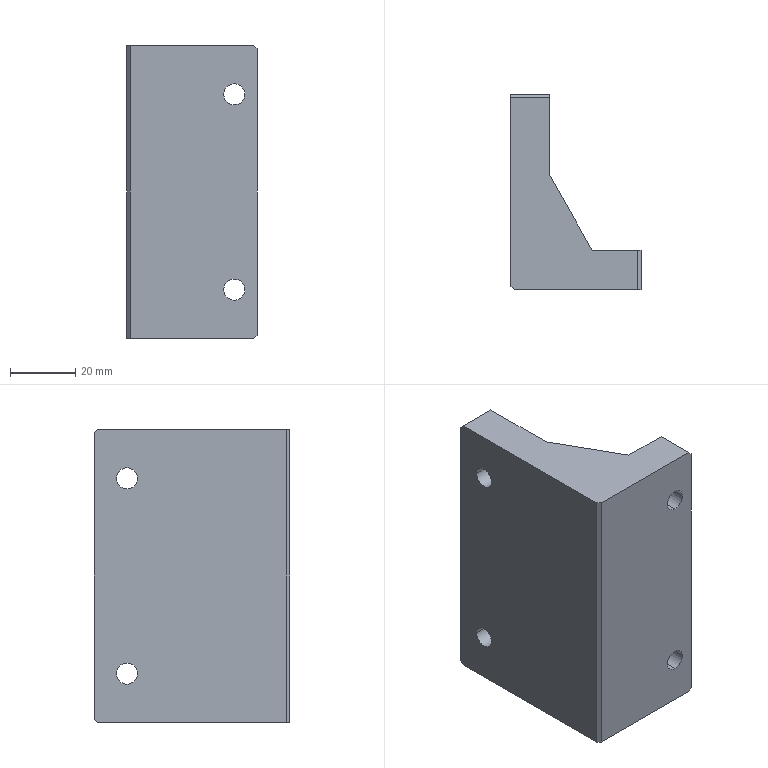Part | NX | features BREP 1 | 1 solid | 22 faces | box 40 x 60 x 90 mm | volume 106833 mm3 | plane 14 | cylinder 8 | commonest cylinder face diameters 6.5 x8
STEP:
#1=CARTESIAN_POINT('',(0.,46.75,75.));
#2=VERTEX_POINT('',#1);
#3=CARTESIAN_POINT('',(0.,53.25,75.));
#4=VERTEX_POINT('',#3);
#5=CARTESIAN_POINT('',(0.,50.,75.));
#6=DIRECTION('',(1.,0.,0.));
#7=DIRECTION('',(0.,0.,-1.));
#8=AXIS2_PLACEMENT_3D('',#5,#6,#7);
#9=CIRCLE('',#8,3.25);
#10=EDGE_CURVE('',#2,#4,#9,.T.);
#11=ORIENTED_EDGE('',*,*,#10,.F.);
#12=CARTESIAN_POINT('',(12.,46.75,75.));
#13=VERTEX_POINT('',#12);
#14=CARTESIAN_POINT('',(-18.,46.75,75.));
#15=DIRECTION('',(1.,0.,0.));
#16=VECTOR('',#15,1000.);
#17=LINE('',#14,#16);
#18=EDGE_CURVE('',#13,#2,#17,.F.);
#19=ORIENTED_EDGE('',*,*,#18,.F.);
#20=CARTESIAN_POINT('',(12.,53.25,75.));
#21=VERTEX_POINT('',#20);
#22=CARTESIAN_POINT('',(12.,50.,75.));
#23=DIRECTION('',(1.,0.,0.));
#24=DIRECTION('',(0.,1.,0.));
#25=AXIS2_PLACEMENT_3D('',#22,#23,#24);
#26=CIRCLE('',#25,3.25);
#27=EDGE_CURVE('',#13,#21,#26,.T.);
#28=ORIENTED_EDGE('',*,*,#27,.T.);
#29=CARTESIAN_POINT('',(-18.,53.25,75.));
#30=DIRECTION('',(1.,0.,0.));
#31=VECTOR('',#30,1000.);
#32=LINE('',#29,#31);
#33=EDGE_CURVE('',#21,#4,#32,.F.);
#34=ORIENTED_EDGE('',*,*,#33,.T.);
#35=EDGE_LOOP('',(#11,#19,#28,#34));
#36=FACE_BOUND('',#35,.T.);
#37=CARTESIAN_POINT('',(-18.,50.,75.));
#38=DIRECTION('',(1.,0.,0.));
#39=DIRECTION('',(0.,1.,0.));
#40=AXIS2_PLACEMENT_3D('',#37,#38,#39);
#41=CYLINDRICAL_SURFACE('',#40,3.25);
#42=ADVANCED_FACE('',(#36),#41,.F.);
#43=CARTESIAN_POINT('',(0.,46.75,15.));
#44=VERTEX_POINT('',#43);
#45=CARTESIAN_POINT('',(0.,53.25,15.));
#46=VERTEX_POINT('',#45);
#47=CARTESIAN_POINT('',(0.,50.,15.));
#48=DIRECTION('',(1.,0.,0.));
#49=DIRECTION('',(0.,0.,-1.));
#50=AXIS2_PLACEMENT_3D('',#47,#48,#49);
#51=CIRCLE('',#50,3.25);
#52=EDGE_CURVE('',#44,#46,#51,.T.);
#53=ORIENTED_EDGE('',*,*,#52,.F.);
#54=CARTESIAN_POINT('',(12.,46.75,15.));
#55=VERTEX_POINT('',#54);
#56=CARTESIAN_POINT('',(-18.,46.75,15.));
#57=DIRECTION('',(1.,0.,0.));
#58=VECTOR('',#57,1000.);
#59=LINE('',#56,#58);
#60=EDGE_CURVE('',#55,#44,#59,.F.);
#61=ORIENTED_EDGE('',*,*,#60,.F.);
#62=CARTESIAN_POINT('',(12.,53.25,15.));
#63=VERTEX_POINT('',#62);
#64=CARTESIAN_POINT('',(12.,50.,15.));
#65=DIRECTION('',(1.,0.,0.));
#66=DIRECTION('',(0.,1.,0.));
#67=AXIS2_PLACEMENT_3D('',#64,#65,#66);
#68=CIRCLE('',#67,3.25);
#69=EDGE_CURVE('',#55,#63,#68,.T.);
#70=ORIENTED_EDGE('',*,*,#69,.T.);
#71=CARTESIAN_POINT('',(-18.,53.25,15.));
#72=DIRECTION('',(1.,0.,0.));
#73=VECTOR('',#72,1000.);
#74=LINE('',#71,#73);
#75=EDGE_CURVE('',#63,#46,#74,.F.);
#76=ORIENTED_EDGE('',*,*,#75,.T.);
#77=EDGE_LOOP('',(#53,#61,#70,#76));
#78=FACE_BOUND('',#77,.T.);
#79=CARTESIAN_POINT('',(-18.,50.,15.));
#80=DIRECTION('',(1.,0.,0.));
#81=DIRECTION('',(0.,1.,0.));
#82=AXIS2_PLACEMENT_3D('',#79,#80,#81);
#83=CYLINDRICAL_SURFACE('',#82,3.25);
#84=ADVANCED_FACE('',(#78),#83,.F.);
#85=CARTESIAN_POINT('',(33.,0.,11.75));
#86=VERTEX_POINT('',#85);
#87=CARTESIAN_POINT('',(33.,0.,18.25));
#88=VERTEX_POINT('',#87);
#89=CARTESIAN_POINT('',(33.,0.,15.));
#90=DIRECTION('',(0.,1.,0.));
#91=DIRECTION('',(0.,0.,1.));
#92=AXIS2_PLACEMENT_3D('',#89,#90,#91);
#93=CIRCLE('',#92,3.25);
#94=EDGE_CURVE('',#86,#88,#93,.T.);
#95=ORIENTED_EDGE('',*,*,#94,.F.);
#96=CARTESIAN_POINT('',(33.,12.,11.75));
#97=VERTEX_POINT('',#96);
#98=CARTESIAN_POINT('',(33.,12.,11.75));
#99=DIRECTION('',(0.,1.,0.));
#100=VECTOR('',#99,1000.);
#101=LINE('',#98,#100);
#102=EDGE_CURVE('',#97,#86,#101,.F.);
#103=ORIENTED_EDGE('',*,*,#102,.F.);
#104=CARTESIAN_POINT('',(33.,12.,18.25));
#105=VERTEX_POINT('',#104);
#106=CARTESIAN_POINT('',(33.,12.,15.));
#107=DIRECTION('',(0.,1.,0.));
#108=DIRECTION('',(0.,0.,1.));
#109=AXIS2_PLACEMENT_3D('',#106,#107,#108);
#110=CIRCLE('',#109,3.25);
#111=EDGE_CURVE('',#97,#105,#110,.T.);
#112=ORIENTED_EDGE('',*,*,#111,.T.);
#113=CARTESIAN_POINT('',(33.,12.,18.25));
#114=DIRECTION('',(0.,1.,0.));
#115=VECTOR('',#114,1000.);
#116=LINE('',#113,#115);
#117=EDGE_CURVE('',#105,#88,#116,.F.);
#118=ORIENTED_EDGE('',*,*,#117,.T.);
#119=EDGE_LOOP('',(#95,#103,#112,#118));
#120=FACE_BOUND('',#119,.T.);
#121=CARTESIAN_POINT('',(33.,12.,15.));
#122=DIRECTION('',(0.,1.,0.));
#123=DIRECTION('',(0.,0.,1.));
#124=AXIS2_PLACEMENT_3D('',#121,#122,#123);
#125=CYLINDRICAL_SURFACE('',#124,3.25);
#126=ADVANCED_FACE('',(#120),#125,.F.);
#127=CARTESIAN_POINT('',(33.,0.,71.75));
#128=VERTEX_POINT('',#127);
#129=CARTESIAN_POINT('',(33.,0.,78.25));
#130=VERTEX_POINT('',#129);
#131=CARTESIAN_POINT('',(33.,0.,75.));
#132=DIRECTION('',(0.,1.,0.));
#133=DIRECTION('',(0.,0.,1.));
#134=AXIS2_PLACEMENT_3D('',#131,#132,#133);
#135=CIRCLE('',#134,3.25);
#136=EDGE_CURVE('',#128,#130,#135,.T.);
#137=ORIENTED_EDGE('',*,*,#136,.F.);
#138=CARTESIAN_POINT('',(33.,12.,71.75));
#139=VERTEX_POINT('',#138);
#140=CARTESIAN_POINT('',(33.,12.,71.75));
#141=DIRECTION('',(0.,1.,0.));
#142=VECTOR('',#141,1000.);
#143=LINE('',#140,#142);
#144=EDGE_CURVE('',#139,#128,#143,.F.);
#145=ORIENTED_EDGE('',*,*,#144,.F.);
#146=CARTESIAN_POINT('',(33.,12.,78.25));
#147=VERTEX_POINT('',#146);
#148=CARTESIAN_POINT('',(33.,12.,75.));
#149=DIRECTION('',(0.,1.,0.));
#150=DIRECTION('',(0.,0.,1.));
#151=AXIS2_PLACEMENT_3D('',#148,#149,#150);
#152=CIRCLE('',#151,3.25);
#153=EDGE_CURVE('',#139,#147,#152,.T.);
#154=ORIENTED_EDGE('',*,*,#153,.T.);
#155=CARTESIAN_POINT('',(33.,12.,78.25));
#156=DIRECTION('',(0.,1.,0.));
#157=VECTOR('',#156,1000.);
#158=LINE('',#155,#157);
#159=EDGE_CURVE('',#147,#130,#158,.F.);
#160=ORIENTED_EDGE('',*,*,#159,.T.);
#161=EDGE_LOOP('',(#137,#145,#154,#160));
#162=FACE_BOUND('',#161,.T.);
#163=CARTESIAN_POINT('',(33.,12.,75.));
#164=DIRECTION('',(0.,1.,0.));
#165=DIRECTION('',(0.,0.,1.));
#166=AXIS2_PLACEMENT_3D('',#163,#164,#165);
#167=CYLINDRICAL_SURFACE('',#166,3.25);
#168=ADVANCED_FACE('',(#162),#167,.F.);
#169=CARTESIAN_POINT('',(1.,0.,90.));
#170=VERTEX_POINT('',#169);
#171=CARTESIAN_POINT('',(39.,0.,90.));
#172=VERTEX_POINT('',#171);
#173=CARTESIAN_POINT('',(40.,0.,90.));
#174=DIRECTION('',(1.,0.,0.));
#175=VECTOR('',#174,1000.);
#176=LINE('',#173,#175);
#177=EDGE_CURVE('',#170,#172,#176,.T.);
#178=ORIENTED_EDGE('',*,*,#177,.F.);
#179=CARTESIAN_POINT('',(1.,0.,0.));
#180=VERTEX_POINT('',#179);
#181=CARTESIAN_POINT('',(1.,0.,90.));
#182=DIRECTION('',(0.,0.,-1.));
#183=VECTOR('',#182,1000.);
#184=LINE('',#181,#183);
#185=EDGE_CURVE('',#170,#180,#184,.T.);
#186=ORIENTED_EDGE('',*,*,#185,.T.);
#187=CARTESIAN_POINT('',(39.,0.,0.));
#188=VERTEX_POINT('',#187);
#189=CARTESIAN_POINT('',(40.,0.,0.));
#190=DIRECTION('',(1.,0.,0.));
#191=VECTOR('',#190,1000.);
#192=LINE('',#189,#191);
#193=EDGE_CURVE('',#180,#188,#192,.T.);
#194=ORIENTED_EDGE('',*,*,#193,.T.);
#195=CARTESIAN_POINT('',(40.,0.,1.));
#196=VERTEX_POINT('',#195);
#197=CARTESIAN_POINT('',(40.,0.,1.));
#198=DIRECTION('',(0.7071,0.,0.7071));
#199=VECTOR('',#198,1000.);
#200=LINE('',#197,#199);
#201=EDGE_CURVE('',#188,#196,#200,.T.);
#202=ORIENTED_EDGE('',*,*,#201,.T.);
#203=CARTESIAN_POINT('',(40.,0.,89.));
#204=VERTEX_POINT('',#203);
#205=CARTESIAN_POINT('',(40.,0.,90.));
#206=DIRECTION('',(0.,0.,-1.));
#207=VECTOR('',#206,1000.);
#208=LINE('',#205,#207);
#209=EDGE_CURVE('',#204,#196,#208,.T.);
#210=ORIENTED_EDGE('',*,*,#209,.F.);
#211=CARTESIAN_POINT('',(39.,0.,90.));
#212=DIRECTION('',(-0.7071,0.,0.7071));
#213=VECTOR('',#212,1000.);
#214=LINE('',#211,#213);
#215=EDGE_CURVE('',#204,#172,#214,.T.);
#216=ORIENTED_EDGE('',*,*,#215,.T.);
#217=EDGE_LOOP('',(#178,#186,#194,#202,#210,#216));
#218=FACE_BOUND('',#217,.T.);
#219=CARTESIAN_POINT('',(33.,0.,15.));
#220=DIRECTION('',(0.,1.,0.));
#221=DIRECTION('',(0.,0.,1.));
#222=AXIS2_PLACEMENT_3D('',#219,#220,#221);
#223=CIRCLE('',#222,3.25);
#224=EDGE_CURVE('',#88,#86,#223,.T.);
#225=ORIENTED_EDGE('',*,*,#224,.T.);
#226=ORIENTED_EDGE('',*,*,#94,.T.);
#227=EDGE_LOOP('',(#225,#226));
#228=FACE_BOUND('',#227,.T.);
#229=CARTESIAN_POINT('',(33.,0.,75.));
#230=DIRECTION('',(0.,1.,0.));
#231=DIRECTION('',(0.,0.,1.));
#232=AXIS2_PLACEMENT_3D('',#229,#230,#231);
#233=CIRCLE('',#232,3.25);
#234=EDGE_CURVE('',#130,#128,#233,.T.);
#235=ORIENTED_EDGE('',*,*,#234,.T.);
#236=ORIENTED_EDGE('',*,*,#136,.T.);
#237=EDGE_LOOP('',(#235,#236));
#238=FACE_BOUND('',#237,.T.);
#239=CARTESIAN_POINT('',(40.,0.,90.));
#240=DIRECTION('',(0.,1.,0.));
#241=DIRECTION('',(1.,0.,0.));
#242=AXIS2_PLACEMENT_3D('',#239,#240,#241);
#243=PLANE('',#242);
#244=ADVANCED_FACE('',(#218,#228,#238),#243,.F.);
#245=ORIENTED_EDGE('',*,*,#209,.T.);
#246=CARTESIAN_POINT('',(40.,12.,1.));
#247=VERTEX_POINT('',#246);
#248=CARTESIAN_POINT('',(40.,12.,1.));
#249=DIRECTION('',(0.,1.,0.));
#250=VECTOR('',#249,1000.);
#251=LINE('',#248,#250);
#252=EDGE_CURVE('',#196,#247,#251,.T.);
#253=ORIENTED_EDGE('',*,*,#252,.T.);
#254=CARTESIAN_POINT('',(40.,12.,89.));
#255=VERTEX_POINT('',#254);
#256=CARTESIAN_POINT('',(40.,12.,90.));
#257=DIRECTION('',(0.,0.,-1.));
#258=VECTOR('',#257,1000.);
#259=LINE('',#256,#258);
#260=EDGE_CURVE('',#255,#247,#259,.T.);
#261=ORIENTED_EDGE('',*,*,#260,.F.);
#262=CARTESIAN_POINT('',(40.,12.,89.));
#263=DIRECTION('',(0.,-1.,0.));
#264=VECTOR('',#263,1000.);
#265=LINE('',#262,#264);
#266=EDGE_CURVE('',#255,#204,#265,.T.);
#267=ORIENTED_EDGE('',*,*,#266,.T.);
#268=EDGE_LOOP('',(#245,#253,#261,#267));
#269=FACE_BOUND('',#268,.T.);
#270=CARTESIAN_POINT('',(40.,12.,90.));
#271=DIRECTION('',(-1.,0.,0.));
#272=DIRECTION('',(0.,0.,1.));
#273=AXIS2_PLACEMENT_3D('',#270,#271,#272);
#274=PLANE('',#273);
#275=ADVANCED_FACE('',(#269),#274,.F.);
#276=ORIENTED_EDGE('',*,*,#260,.T.);
#277=CARTESIAN_POINT('',(39.,12.,0.));
#278=VERTEX_POINT('',#277);
#279=CARTESIAN_POINT('',(40.,12.,1.));
#280=DIRECTION('',(-0.7071,0.,-0.7071));
#281=VECTOR('',#280,1000.);
#282=LINE('',#279,#281);
#283=EDGE_CURVE('',#247,#278,#282,.T.);
#284=ORIENTED_EDGE('',*,*,#283,.T.);
#285=CARTESIAN_POINT('',(25.,12.,0.));
#286=VERTEX_POINT('',#285);
#287=CARTESIAN_POINT('',(25.,12.,0.));
#288=DIRECTION('',(-1.,0.,0.));
#289=VECTOR('',#288,1000.);
#290=LINE('',#287,#289);
#291=EDGE_CURVE('',#278,#286,#290,.T.);
#292=ORIENTED_EDGE('',*,*,#291,.T.);
#293=CARTESIAN_POINT('',(25.,12.,90.));
#294=VERTEX_POINT('',#293);
#295=CARTESIAN_POINT('',(25.,12.,90.));
#296=DIRECTION('',(0.,0.,-1.));
#297=VECTOR('',#296,1000.);
#298=LINE('',#295,#297);
#299=EDGE_CURVE('',#294,#286,#298,.T.);
#300=ORIENTED_EDGE('',*,*,#299,.F.);
#301=CARTESIAN_POINT('',(39.,12.,90.));
#302=VERTEX_POINT('',#301);
#303=CARTESIAN_POINT('',(25.,12.,90.));
#304=DIRECTION('',(-1.,0.,0.));
#305=VECTOR('',#304,1000.);
#306=LINE('',#303,#305);
#307=EDGE_CURVE('',#302,#294,#306,.T.);
#308=ORIENTED_EDGE('',*,*,#307,.F.);
#309=CARTESIAN_POINT('',(39.,12.,90.));
#310=DIRECTION('',(0.7071,0.,-0.7071));
#311=VECTOR('',#310,1000.);
#312=LINE('',#309,#311);
#313=EDGE_CURVE('',#302,#255,#312,.T.);
#314=ORIENTED_EDGE('',*,*,#313,.T.);
#315=EDGE_LOOP('',(#276,#284,#292,#300,#308,#314));
#316=FACE_BOUND('',#315,.T.);
#317=CARTESIAN_POINT('',(33.,12.,15.));
#318=DIRECTION('',(0.,1.,0.));
#319=DIRECTION('',(0.,0.,1.));
#320=AXIS2_PLACEMENT_3D('',#317,#318,#319);
#321=CIRCLE('',#320,3.25);
#322=EDGE_CURVE('',#105,#97,#321,.T.);
#323=ORIENTED_EDGE('',*,*,#322,.F.);
#324=ORIENTED_EDGE('',*,*,#111,.F.);
#325=EDGE_LOOP('',(#323,#324));
#326=FACE_BOUND('',#325,.T.);
#327=CARTESIAN_POINT('',(33.,12.,75.));
#328=DIRECTION('',(0.,1.,0.));
#329=DIRECTION('',(0.,0.,1.));
#330=AXIS2_PLACEMENT_3D('',#327,#328,#329);
#331=CIRCLE('',#330,3.25);
#332=EDGE_CURVE('',#147,#139,#331,.T.);
#333=ORIENTED_EDGE('',*,*,#332,.F.);
#334=ORIENTED_EDGE('',*,*,#153,.F.);
#335=EDGE_LOOP('',(#333,#334));
#336=FACE_BOUND('',#335,.T.);
#337=CARTESIAN_POINT('',(25.,12.,90.));
#338=DIRECTION('',(0.,-1.,0.));
#339=DIRECTION('',(0.,0.,-1.));
#340=AXIS2_PLACEMENT_3D('',#337,#338,#339);
#341=PLANE('',#340);
#342=ADVANCED_FACE('',(#316,#326,#336),#341,.F.);
#343=CARTESIAN_POINT('',(12.,35.,0.));
#344=VERTEX_POINT('',#343);
#345=CARTESIAN_POINT('',(12.,35.,0.));
#346=DIRECTION('',(-0.4921,0.8706,0.));
#347=VECTOR('',#346,1000.);
#348=LINE('',#345,#347);
#349=EDGE_CURVE('',#286,#344,#348,.T.);
#350=ORIENTED_EDGE('',*,*,#349,.T.);
#351=CARTESIAN_POINT('',(12.,35.,90.));
#352=VERTEX_POINT('',#351);
#353=CARTESIAN_POINT('',(12.,35.,90.));
#354=DIRECTION('',(0.,0.,-1.));
#355=VECTOR('',#354,1000.);
#356=LINE('',#353,#355);
#357=EDGE_CURVE('',#352,#344,#356,.T.);
#358=ORIENTED_EDGE('',*,*,#357,.F.);
#359=CARTESIAN_POINT('',(12.,35.,90.));
#360=DIRECTION('',(-0.4921,0.8706,0.));
#361=VECTOR('',#360,1000.);
#362=LINE('',#359,#361);
#363=EDGE_CURVE('',#294,#352,#362,.T.);
#364=ORIENTED_EDGE('',*,*,#363,.F.);
#365=ORIENTED_EDGE('',*,*,#299,.T.);
#366=EDGE_LOOP('',(#350,#358,#364,#365));
#367=FACE_BOUND('',#366,.T.);
#368=CARTESIAN_POINT('',(12.,35.,90.));
#369=DIRECTION('',(-0.8706,-0.4921,0.));
#370=DIRECTION('',(-0.4921,0.8706,0.));
#371=AXIS2_PLACEMENT_3D('',#368,#369,#370);
#372=PLANE('',#371);
#373=ADVANCED_FACE('',(#367),#372,.F.);
#374=CARTESIAN_POINT('',(12.,60.,89.));
#375=VERTEX_POINT('',#374);
#376=CARTESIAN_POINT('',(12.,60.,1.));
#377=VERTEX_POINT('',#376);
#378=CARTESIAN_POINT('',(12.,60.,90.));
#379=DIRECTION('',(0.,0.,-1.));
#380=VECTOR('',#379,1000.);
#381=LINE('',#378,#380);
#382=EDGE_CURVE('',#375,#377,#381,.T.);
#383=ORIENTED_EDGE('',*,*,#382,.F.);
#384=CARTESIAN_POINT('',(12.,59.,90.));
#385=VERTEX_POINT('',#384);
#386=CARTESIAN_POINT('',(12.,59.,90.));
#387=DIRECTION('',(0.,-0.7071,0.7071));
#388=VECTOR('',#387,1000.);
#389=LINE('',#386,#388);
#390=EDGE_CURVE('',#375,#385,#389,.T.);
#391=ORIENTED_EDGE('',*,*,#390,.T.);
#392=CARTESIAN_POINT('',(12.,60.,90.));
#393=DIRECTION('',(0.,1.,0.));
#394=VECTOR('',#393,1000.);
#395=LINE('',#392,#394);
#396=EDGE_CURVE('',#352,#385,#395,.T.);
#397=ORIENTED_EDGE('',*,*,#396,.F.);
#398=ORIENTED_EDGE('',*,*,#357,.T.);
#399=CARTESIAN_POINT('',(12.,59.,0.));
#400=VERTEX_POINT('',#399);
#401=CARTESIAN_POINT('',(12.,60.,0.));
#402=DIRECTION('',(0.,1.,0.));
#403=VECTOR('',#402,1000.);
#404=LINE('',#401,#403);
#405=EDGE_CURVE('',#344,#400,#404,.T.);
#406=ORIENTED_EDGE('',*,*,#405,.T.);
#407=CARTESIAN_POINT('',(12.,60.,1.));
#408=DIRECTION('',(0.,0.7071,0.7071));
#409=VECTOR('',#408,1000.);
#410=LINE('',#407,#409);
#411=EDGE_CURVE('',#400,#377,#410,.T.);
#412=ORIENTED_EDGE('',*,*,#411,.T.);
#413=EDGE_LOOP('',(#383,#391,#397,#398,#406,#412));
#414=FACE_BOUND('',#413,.T.);
#415=CARTESIAN_POINT('',(12.,50.,75.));
#416=DIRECTION('',(1.,0.,0.));
#417=DIRECTION('',(0.,1.,0.));
#418=AXIS2_PLACEMENT_3D('',#415,#416,#417);
#419=CIRCLE('',#418,3.25);
#420=EDGE_CURVE('',#21,#13,#419,.T.);
#421=ORIENTED_EDGE('',*,*,#420,.F.);
#422=ORIENTED_EDGE('',*,*,#27,.F.);
#423=EDGE_LOOP('',(#421,#422));
#424=FACE_BOUND('',#423,.T.);
#425=CARTESIAN_POINT('',(12.,50.,15.));
#426=DIRECTION('',(1.,0.,0.));
#427=DIRECTION('',(0.,1.,0.));
#428=AXIS2_PLACEMENT_3D('',#425,#426,#427);
#429=CIRCLE('',#428,3.25);
#430=EDGE_CURVE('',#63,#55,#429,.T.);
#431=ORIENTED_EDGE('',*,*,#430,.F.);
#432=ORIENTED_EDGE('',*,*,#69,.F.);
#433=EDGE_LOOP('',(#431,#432));
#434=FACE_BOUND('',#433,.T.);
#435=CARTESIAN_POINT('',(12.,60.,90.));
#436=DIRECTION('',(-1.,0.,0.));
#437=DIRECTION('',(0.,1.,0.));
#438=AXIS2_PLACEMENT_3D('',#435,#436,#437);
#439=PLANE('',#438);
#440=ADVANCED_FACE('',(#414,#424,#434),#439,.F.);
#441=CARTESIAN_POINT('',(0.,60.,89.));
#442=VERTEX_POINT('',#441);
#443=CARTESIAN_POINT('',(0.,60.,1.));
#444=VERTEX_POINT('',#443);
#445=CARTESIAN_POINT('',(0.,60.,90.));
#446=DIRECTION('',(0.,0.,-1.));
#447=VECTOR('',#446,1000.);
#448=LINE('',#445,#447);
#449=EDGE_CURVE('',#442,#444,#448,.T.);
#450=ORIENTED_EDGE('',*,*,#449,.F.);
#451=CARTESIAN_POINT('',(0.,60.,89.));
#452=DIRECTION('',(1.,0.,0.));
#453=VECTOR('',#452,1000.);
#454=LINE('',#451,#453);
#455=EDGE_CURVE('',#442,#375,#454,.T.);
#456=ORIENTED_EDGE('',*,*,#455,.T.);
#457=ORIENTED_EDGE('',*,*,#382,.T.);
#458=CARTESIAN_POINT('',(0.,60.,1.));
#459=DIRECTION('',(-1.,0.,0.));
#460=VECTOR('',#459,1000.);
#461=LINE('',#458,#460);
#462=EDGE_CURVE('',#377,#444,#461,.T.);
#463=ORIENTED_EDGE('',*,*,#462,.T.);
#464=EDGE_LOOP('',(#450,#456,#457,#463));
#465=FACE_BOUND('',#464,.T.);
#466=CARTESIAN_POINT('',(0.,60.,90.));
#467=DIRECTION('',(0.,-1.,0.));
#468=DIRECTION('',(0.,0.,-1.));
#469=AXIS2_PLACEMENT_3D('',#466,#467,#468);
#470=PLANE('',#469);
#471=ADVANCED_FACE('',(#465),#470,.F.);
#472=CARTESIAN_POINT('',(0.,59.,0.));
#473=VERTEX_POINT('',#472);
#474=CARTESIAN_POINT('',(0.,1.,0.));
#475=VERTEX_POINT('',#474);
#476=CARTESIAN_POINT('',(0.,0.,0.));
#477=DIRECTION('',(0.,-1.,0.));
#478=VECTOR('',#477,1000.);
#479=LINE('',#476,#478);
#480=EDGE_CURVE('',#473,#475,#479,.T.);
#481=ORIENTED_EDGE('',*,*,#480,.T.);
#482=CARTESIAN_POINT('',(0.,1.,90.));
#483=VERTEX_POINT('',#482);
#484=CARTESIAN_POINT('',(0.,1.,90.));
#485=DIRECTION('',(0.,0.,1.));
#486=VECTOR('',#485,1000.);
#487=LINE('',#484,#486);
#488=EDGE_CURVE('',#475,#483,#487,.T.);
#489=ORIENTED_EDGE('',*,*,#488,.T.);
#490=CARTESIAN_POINT('',(0.,59.,90.));
#491=VERTEX_POINT('',#490);
#492=CARTESIAN_POINT('',(0.,0.,90.));
#493=DIRECTION('',(0.,-1.,0.));
#494=VECTOR('',#493,1000.);
#495=LINE('',#492,#494);
#496=EDGE_CURVE('',#491,#483,#495,.T.);
#497=ORIENTED_EDGE('',*,*,#496,.F.);
#498=CARTESIAN_POINT('',(0.,59.,90.));
#499=DIRECTION('',(0.,0.7071,-0.7071));
#500=VECTOR('',#499,1000.);
#501=LINE('',#498,#500);
#502=EDGE_CURVE('',#491,#442,#501,.T.);
#503=ORIENTED_EDGE('',*,*,#502,.T.);
#504=ORIENTED_EDGE('',*,*,#449,.T.);
#505=CARTESIAN_POINT('',(0.,60.,1.));
#506=DIRECTION('',(0.,-0.7071,-0.7071));
#507=VECTOR('',#506,1000.);
#508=LINE('',#505,#507);
#509=EDGE_CURVE('',#444,#473,#508,.T.);
#510=ORIENTED_EDGE('',*,*,#509,.T.);
#511=EDGE_LOOP('',(#481,#489,#497,#503,#504,#510));
#512=FACE_BOUND('',#511,.T.);
#513=CARTESIAN_POINT('',(0.,50.,75.));
#514=DIRECTION('',(1.,0.,0.));
#515=DIRECTION('',(0.,0.,-1.));
#516=AXIS2_PLACEMENT_3D('',#513,#514,#515);
#517=CIRCLE('',#516,3.25);
#518=EDGE_CURVE('',#4,#2,#517,.T.);
#519=ORIENTED_EDGE('',*,*,#518,.T.);
#520=ORIENTED_EDGE('',*,*,#10,.T.);
#521=EDGE_LOOP('',(#519,#520));
#522=FACE_BOUND('',#521,.T.);
#523=CARTESIAN_POINT('',(0.,50.,15.));
#524=DIRECTION('',(1.,0.,0.));
#525=DIRECTION('',(0.,0.,-1.));
#526=AXIS2_PLACEMENT_3D('',#523,#524,#525);
#527=CIRCLE('',#526,3.25);
#528=EDGE_CURVE('',#46,#44,#527,.T.);
#529=ORIENTED_EDGE('',*,*,#528,.T.);
#530=ORIENTED_EDGE('',*,*,#52,.T.);
#531=EDGE_LOOP('',(#529,#530));
#532=FACE_BOUND('',#531,.T.);
#533=CARTESIAN_POINT('',(0.,0.,90.));
#534=DIRECTION('',(1.,0.,0.));
#535=DIRECTION('',(0.,1.,0.));
#536=AXIS2_PLACEMENT_3D('',#533,#534,#535);
#537=PLANE('',#536);
#538=ADVANCED_FACE('',(#512,#522,#532),#537,.F.);
#539=ORIENTED_EDGE('',*,*,#496,.T.);
#540=CARTESIAN_POINT('',(1.,0.,90.));
#541=DIRECTION('',(0.7071,-0.7071,0.));
#542=VECTOR('',#541,1000.);
#543=LINE('',#540,#542);
#544=EDGE_CURVE('',#483,#170,#543,.T.);
#545=ORIENTED_EDGE('',*,*,#544,.T.);
#546=ORIENTED_EDGE('',*,*,#177,.T.);
#547=CARTESIAN_POINT('',(39.,0.,90.));
#548=DIRECTION('',(0.,1.,0.));
#549=VECTOR('',#548,1000.);
#550=LINE('',#547,#549);
#551=EDGE_CURVE('',#172,#302,#550,.T.);
#552=ORIENTED_EDGE('',*,*,#551,.T.);
#553=ORIENTED_EDGE('',*,*,#307,.T.);
#554=ORIENTED_EDGE('',*,*,#363,.T.);
#555=ORIENTED_EDGE('',*,*,#396,.T.);
#556=CARTESIAN_POINT('',(0.,59.,90.));
#557=DIRECTION('',(-1.,0.,0.));
#558=VECTOR('',#557,1000.);
#559=LINE('',#556,#558);
#560=EDGE_CURVE('',#385,#491,#559,.T.);
#561=ORIENTED_EDGE('',*,*,#560,.T.);
#562=EDGE_LOOP('',(#539,#545,#546,#552,#553,#554,#555,#561));
#563=FACE_BOUND('',#562,.T.);
#564=CARTESIAN_POINT('',(0.,0.,90.));
#565=DIRECTION('',(0.,0.,-1.));
#566=DIRECTION('',(0.,-1.,0.));
#567=AXIS2_PLACEMENT_3D('',#564,#565,#566);
#568=PLANE('',#567);
#569=ADVANCED_FACE('',(#563),#568,.F.);
#570=ORIENTED_EDGE('',*,*,#193,.F.);
#571=CARTESIAN_POINT('',(0.5,0.5,0.));
#572=DIRECTION('',(-0.7071,0.7071,0.));
#573=VECTOR('',#572,1000.);
#574=LINE('',#571,#573);
#575=EDGE_CURVE('',#180,#475,#574,.T.);
#576=ORIENTED_EDGE('',*,*,#575,.T.);
#577=ORIENTED_EDGE('',*,*,#480,.F.);
#578=CARTESIAN_POINT('',(12.,59.,0.));
#579=DIRECTION('',(1.,0.,0.));
#580=VECTOR('',#579,1000.);
#581=LINE('',#578,#580);
#582=EDGE_CURVE('',#473,#400,#581,.T.);
#583=ORIENTED_EDGE('',*,*,#582,.T.);
#584=ORIENTED_EDGE('',*,*,#405,.F.);
#585=ORIENTED_EDGE('',*,*,#349,.F.);
#586=ORIENTED_EDGE('',*,*,#291,.F.);
#587=CARTESIAN_POINT('',(39.,0.,0.));
#588=DIRECTION('',(0.,-1.,0.));
#589=VECTOR('',#588,1000.);
#590=LINE('',#587,#589);
#591=EDGE_CURVE('',#278,#188,#590,.T.);
#592=ORIENTED_EDGE('',*,*,#591,.T.);
#593=EDGE_LOOP('',(#570,#576,#577,#583,#584,#585,#586,#592));
#594=FACE_BOUND('',#593,.T.);
#595=CARTESIAN_POINT('',(0.,0.,0.));
#596=DIRECTION('',(0.,0.,-1.));
#597=DIRECTION('',(0.,-1.,0.));
#598=AXIS2_PLACEMENT_3D('',#595,#596,#597);
#599=PLANE('',#598);
#600=ADVANCED_FACE('',(#594),#599,.T.);
#601=ORIENTED_EDGE('',*,*,#201,.F.);
#602=ORIENTED_EDGE('',*,*,#591,.F.);
#603=ORIENTED_EDGE('',*,*,#283,.F.);
#604=ORIENTED_EDGE('',*,*,#252,.F.);
#605=EDGE_LOOP('',(#601,#602,#603,#604));
#606=FACE_BOUND('',#605,.T.);
#607=CARTESIAN_POINT('',(40.,12.,1.));
#608=DIRECTION('',(0.7071,0.,-0.7071));
#609=DIRECTION('',(0.,-1.,0.));
#610=AXIS2_PLACEMENT_3D('',#607,#608,#609);
#611=PLANE('',#610);
#612=ADVANCED_FACE('',(#606),#611,.T.);
#613=ORIENTED_EDGE('',*,*,#215,.F.);
#614=ORIENTED_EDGE('',*,*,#266,.F.);
#615=ORIENTED_EDGE('',*,*,#313,.F.);
#616=ORIENTED_EDGE('',*,*,#551,.F.);
#617=EDGE_LOOP('',(#613,#614,#615,#616));
#618=FACE_BOUND('',#617,.T.);
#619=CARTESIAN_POINT('',(39.,0.,90.));
#620=DIRECTION('',(-0.7071,0.,-0.7071));
#621=DIRECTION('',(-0.7071,0.,0.7071));
#622=AXIS2_PLACEMENT_3D('',#619,#620,#621);
#623=PLANE('',#622);
#624=ADVANCED_FACE('',(#618),#623,.F.);
#625=ORIENTED_EDGE('',*,*,#390,.F.);
#626=ORIENTED_EDGE('',*,*,#455,.F.);
#627=ORIENTED_EDGE('',*,*,#502,.F.);
#628=ORIENTED_EDGE('',*,*,#560,.F.);
#629=EDGE_LOOP('',(#625,#626,#627,#628));
#630=FACE_BOUND('',#629,.T.);
#631=CARTESIAN_POINT('',(0.,59.,90.));
#632=DIRECTION('',(0.,-0.7071,-0.7071));
#633=DIRECTION('',(0.,0.7071,-0.7071));
#634=AXIS2_PLACEMENT_3D('',#631,#632,#633);
#635=PLANE('',#634);
#636=ADVANCED_FACE('',(#630),#635,.F.);
#637=ORIENTED_EDGE('',*,*,#411,.F.);
#638=ORIENTED_EDGE('',*,*,#582,.F.);
#639=ORIENTED_EDGE('',*,*,#509,.F.);
#640=ORIENTED_EDGE('',*,*,#462,.F.);
#641=EDGE_LOOP('',(#637,#638,#639,#640));
#642=FACE_BOUND('',#641,.T.);
#643=CARTESIAN_POINT('',(0.,60.,1.));
#644=DIRECTION('',(0.,0.7071,-0.7071));
#645=DIRECTION('',(-1.,0.,0.));
#646=AXIS2_PLACEMENT_3D('',#643,#644,#645);
#647=PLANE('',#646);
#648=ADVANCED_FACE('',(#642),#647,.T.);
#649=ORIENTED_EDGE('',*,*,#144,.T.);
#650=ORIENTED_EDGE('',*,*,#234,.F.);
#651=ORIENTED_EDGE('',*,*,#159,.F.);
#652=ORIENTED_EDGE('',*,*,#332,.T.);
#653=EDGE_LOOP('',(#649,#650,#651,#652));
#654=FACE_BOUND('',#653,.T.);
#655=CARTESIAN_POINT('',(33.,12.,75.));
#656=DIRECTION('',(0.,1.,0.));
#657=DIRECTION('',(0.,0.,1.));
#658=AXIS2_PLACEMENT_3D('',#655,#656,#657);
#659=CYLINDRICAL_SURFACE('',#658,3.25);
#660=ADVANCED_FACE('',(#654),#659,.F.);
#661=ORIENTED_EDGE('',*,*,#102,.T.);
#662=ORIENTED_EDGE('',*,*,#224,.F.);
#663=ORIENTED_EDGE('',*,*,#117,.F.);
#664=ORIENTED_EDGE('',*,*,#322,.T.);
#665=EDGE_LOOP('',(#661,#662,#663,#664));
#666=FACE_BOUND('',#665,.T.);
#667=CARTESIAN_POINT('',(33.,12.,15.));
#668=DIRECTION('',(0.,1.,0.));
#669=DIRECTION('',(0.,0.,1.));
#670=AXIS2_PLACEMENT_3D('',#667,#668,#669);
#671=CYLINDRICAL_SURFACE('',#670,3.25);
#672=ADVANCED_FACE('',(#666),#671,.F.);
#673=ORIENTED_EDGE('',*,*,#60,.T.);
#674=ORIENTED_EDGE('',*,*,#528,.F.);
#675=ORIENTED_EDGE('',*,*,#75,.F.);
#676=ORIENTED_EDGE('',*,*,#430,.T.);
#677=EDGE_LOOP('',(#673,#674,#675,#676));
#678=FACE_BOUND('',#677,.T.);
#679=CARTESIAN_POINT('',(-18.,50.,15.));
#680=DIRECTION('',(1.,0.,0.));
#681=DIRECTION('',(0.,1.,0.));
#682=AXIS2_PLACEMENT_3D('',#679,#680,#681);
#683=CYLINDRICAL_SURFACE('',#682,3.25);
#684=ADVANCED_FACE('',(#678),#683,.F.);
#685=ORIENTED_EDGE('',*,*,#18,.T.);
#686=ORIENTED_EDGE('',*,*,#518,.F.);
#687=ORIENTED_EDGE('',*,*,#33,.F.);
#688=ORIENTED_EDGE('',*,*,#420,.T.);
#689=EDGE_LOOP('',(#685,#686,#687,#688));
#690=FACE_BOUND('',#689,.T.);
#691=CARTESIAN_POINT('',(-18.,50.,75.));
#692=DIRECTION('',(1.,0.,0.));
#693=DIRECTION('',(0.,1.,0.));
#694=AXIS2_PLACEMENT_3D('',#691,#692,#693);
#695=CYLINDRICAL_SURFACE('',#694,3.25);
#696=ADVANCED_FACE('',(#690),#695,.F.);
#697=ORIENTED_EDGE('',*,*,#544,.F.);
#698=ORIENTED_EDGE('',*,*,#488,.F.);
#699=ORIENTED_EDGE('',*,*,#575,.F.);
#700=ORIENTED_EDGE('',*,*,#185,.F.);
#701=EDGE_LOOP('',(#697,#698,#699,#700));
#702=FACE_BOUND('',#701,.T.);
#703=CARTESIAN_POINT('',(1.,0.,90.));
#704=DIRECTION('',(0.7071,0.7071,0.));
#705=DIRECTION('',(0.,0.,-1.));
#706=AXIS2_PLACEMENT_3D('',#703,#704,#705);
#707=PLANE('',#706);
#708=ADVANCED_FACE('',(#702),#707,.F.);
#709=CLOSED_SHELL('',(#42,#84,#126,#168,#244,#275,#342,#373,#440,#471,#538,#569,#600,#612,#624,#636,#648,#660,#672,#684,#696,#708));
#710=MANIFOLD_SOLID_BREP('',#709);
#711=(LENGTH_UNIT()NAMED_UNIT(*)SI_UNIT(.MILLI.,.METRE.));
#712=UNCERTAINTY_MEASURE_WITH_UNIT(LENGTH_MEASURE(0.00001),#711,'','');
#713=(NAMED_UNIT(*)PLANE_ANGLE_UNIT()SI_UNIT($,.RADIAN.));
#714=(NAMED_UNIT(*)SI_UNIT($,.STERADIAN.)SOLID_ANGLE_UNIT());
#715=(GEOMETRIC_REPRESENTATION_CONTEXT(3)GLOBAL_UNCERTAINTY_ASSIGNED_CONTEXT((#712))GLOBAL_UNIT_ASSIGNED_CONTEXT((#711,#713,#714))REPRESENTATION_CONTEXT('',''));
#716=ADVANCED_BREP_SHAPE_REPRESENTATION('',(#710),#715);